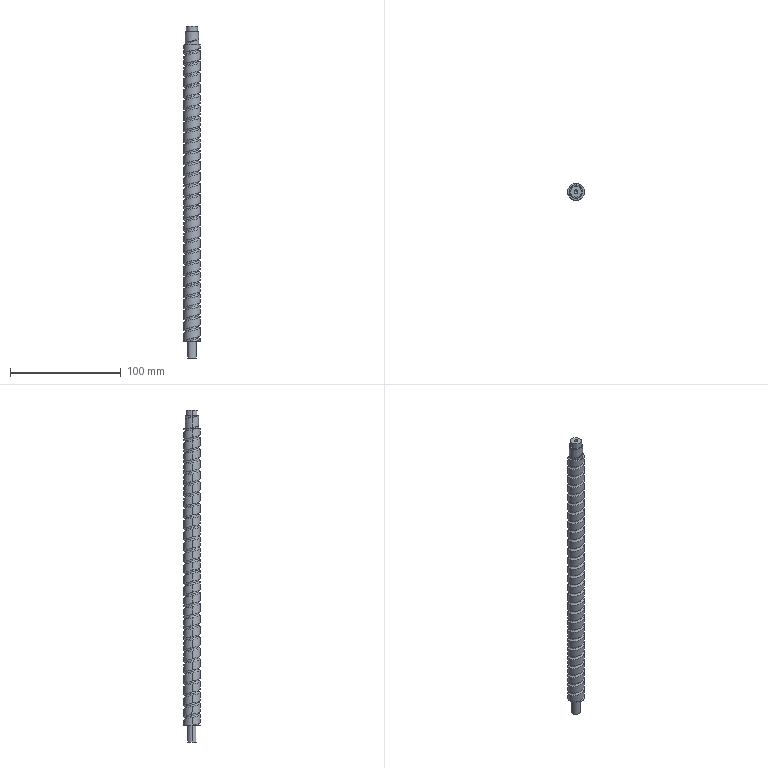Part | STEP file | 300 Lead screw | 1 solid | 77 faces | box 15 x 15 x 300 mm | volume 45152 mm3 | cylinder 68 | plane 5 | cone 2 | spline 2 | commonest cylinder face diameters 15 x56 12 x6 3.3 x2 8 x2 10 x2